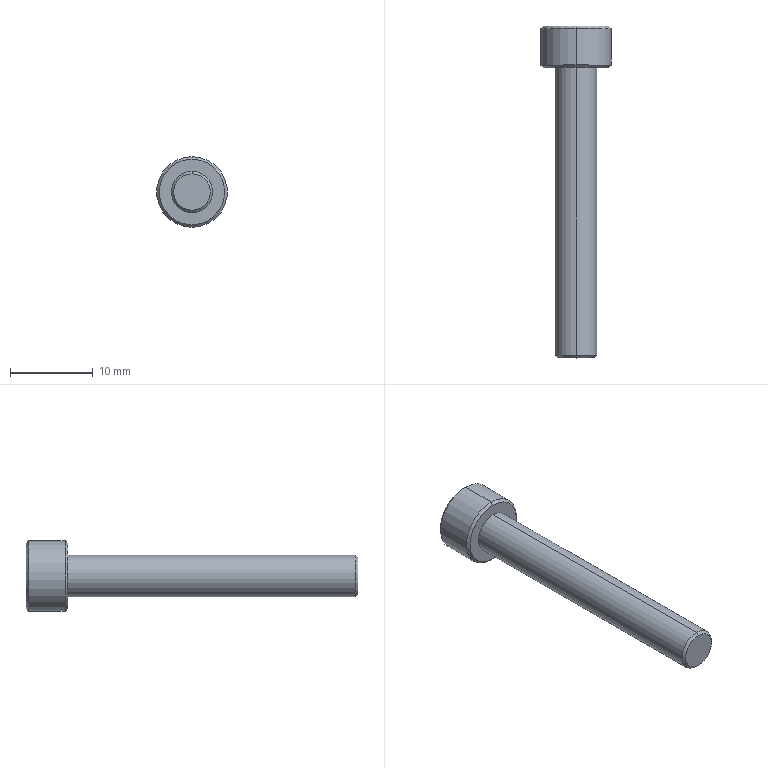Part | STEP file | Hex socket screw M5×35 | 1 solid | 28 faces | box 8.5 x 40 x 8.5 mm | volume 924.588 mm3 | plane 10 | cone 8 | spline 6 | cylinder 4 | commonest cylinder face diameters 5 x2 8.5 x2